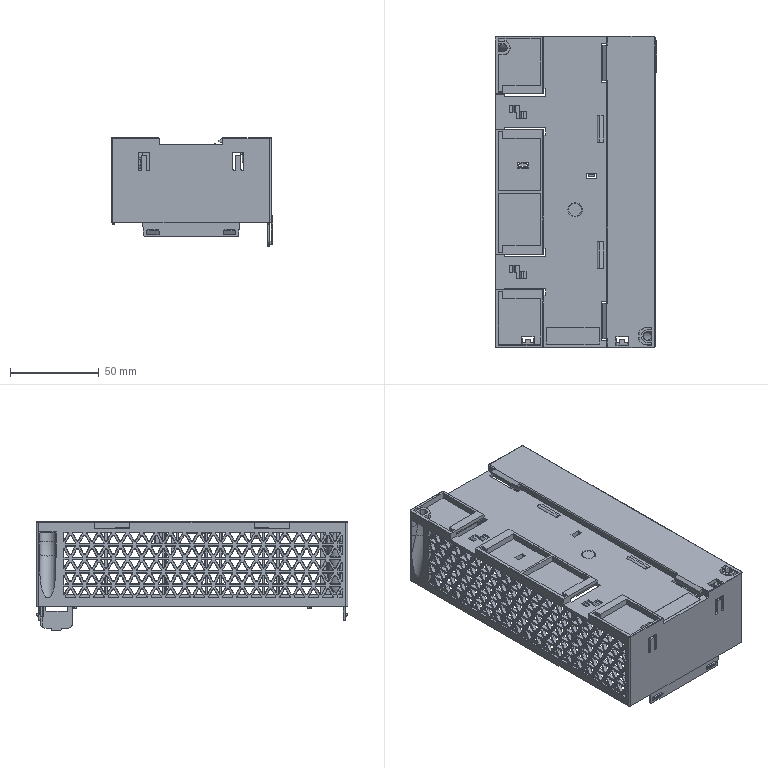Part | Creo | 1 solid | 4053 faces | volume 76793 mm3 | spline 1542 | plane 1408 | cone 823 | cylinder 246 | torus 20 | sphere 10 | other 4 | commonest cylinder face diameters 0.603 x93 0.402 x58 1.005 x41 2.01 x14 5.025 x4 5.226 x4